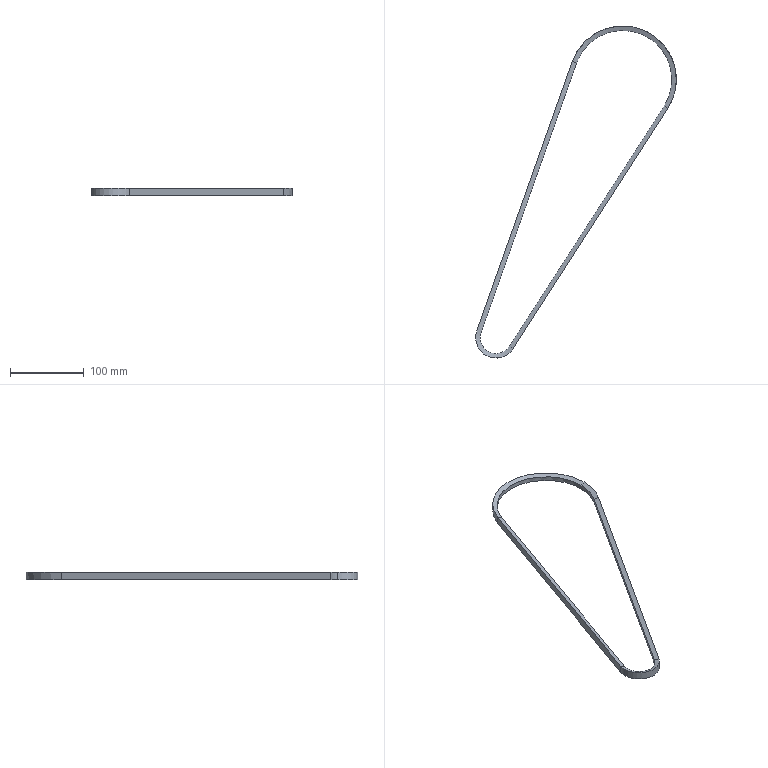Part | SolidWorks | features BaseBody 1 | 1 solid | 20 faces | box 271.5 x 449.339 x 10.319 mm | volume 52741 mm3 | plane 8 | cylinder 6 | cone 6 | commonest cylinder face diameters 42.997 x2 54.997 x2 132.997 x1 144.997 x1
STEP:
#1=CARTESIAN_POINT('',(-148.385,-364.233,5.159));
#2=VERTEX_POINT('',#1);
#3=CARTESIAN_POINT('',(-199.001,-349.342,5.159));
#4=VERTEX_POINT('',#3);
#5=CARTESIAN_POINT('',(-171.503,-349.342,5.159));
#6=DIRECTION('',(0.,0.,-1.));
#7=DIRECTION('',(-1.,0.,0.));
#8=AXIS2_PLACEMENT_3D('',#5,#6,#7);
#9=CIRCLE('',#8,27.499);
#10=EDGE_CURVE('',#2,#4,#9,.T.);
#11=ORIENTED_EDGE('',*,*,#10,.T.);
#12=CARTESIAN_POINT('',(-199.001,-349.342,-5.159));
#13=VERTEX_POINT('',#12);
#14=CARTESIAN_POINT('',(-199.001,-349.342,0.));
#15=DIRECTION('',(0.,0.,-1.));
#16=VECTOR('',#15,1000.);
#17=LINE('',#14,#16);
#18=EDGE_CURVE('',#4,#13,#17,.T.);
#19=ORIENTED_EDGE('',*,*,#18,.T.);
#20=CARTESIAN_POINT('',(-148.385,-364.233,-5.159));
#21=VERTEX_POINT('',#20);
#22=CARTESIAN_POINT('',(-171.503,-349.342,-5.159));
#23=DIRECTION('',(0.,0.,1.));
#24=DIRECTION('',(-1.,0.,0.));
#25=AXIS2_PLACEMENT_3D('',#22,#23,#24);
#26=CIRCLE('',#25,27.499);
#27=EDGE_CURVE('',#13,#21,#26,.T.);
#28=ORIENTED_EDGE('',*,*,#27,.T.);
#29=CARTESIAN_POINT('',(-148.385,-364.233,5.159));
#30=DIRECTION('',(0.,0.,-1.));
#31=VECTOR('',#30,1000.);
#32=LINE('',#29,#31);
#33=EDGE_CURVE('',#2,#21,#32,.T.);
#34=ORIENTED_EDGE('',*,*,#33,.F.);
#35=EDGE_LOOP('',(#11,#19,#28,#34));
#36=FACE_OUTER_BOUND('',#35,.T.);
#37=CARTESIAN_POINT('',(-171.503,-349.342,0.));
#38=DIRECTION('',(0.,0.,-1.));
#39=DIRECTION('',(-1.,0.,0.));
#40=AXIS2_PLACEMENT_3D('',#37,#38,#39);
#41=CYLINDRICAL_SURFACE('',#40,27.499);
#42=ADVANCED_FACE('',(#36),#41,.T.);
#43=CARTESIAN_POINT('',(66.499,0.,2.976));
#44=VERTEX_POINT('',#43);
#45=CARTESIAN_POINT('',(-62.681,22.206,2.976));
#46=VERTEX_POINT('',#45);
#47=CARTESIAN_POINT('',(0.,0.,2.976));
#48=DIRECTION('',(0.,0.,1.));
#49=DIRECTION('',(-0.8407,0.5415,0.));
#50=AXIS2_PLACEMENT_3D('',#47,#48,#49);
#51=CIRCLE('',#50,66.499);
#52=EDGE_CURVE('',#44,#46,#51,.T.);
#53=ORIENTED_EDGE('',*,*,#52,.F.);
#54=CARTESIAN_POINT('',(72.499,0.,5.159));
#55=VERTEX_POINT('',#54);
#56=CARTESIAN_POINT('',(72.499,0.,5.159));
#57=DIRECTION('',(0.9397,0.,0.342));
#58=VECTOR('',#57,1000.);
#59=LINE('',#56,#58);
#60=EDGE_CURVE('',#44,#55,#59,.T.);
#61=ORIENTED_EDGE('',*,*,#60,.T.);
#62=CARTESIAN_POINT('',(-68.337,24.21,5.159));
#63=VERTEX_POINT('',#62);
#64=CARTESIAN_POINT('',(0.,0.,5.159));
#65=DIRECTION('',(0.,0.,-1.));
#66=DIRECTION('',(-1.,0.,0.));
#67=AXIS2_PLACEMENT_3D('',#64,#65,#66);
#68=CIRCLE('',#67,72.499);
#69=EDGE_CURVE('',#63,#55,#68,.T.);
#70=ORIENTED_EDGE('',*,*,#69,.F.);
#71=CARTESIAN_POINT('',(-65.509,23.208,4.068));
#72=DIRECTION('',(-0.8858,0.3138,0.342));
#73=VECTOR('',#72,1000.);
#74=LINE('',#71,#73);
#75=EDGE_CURVE('',#46,#63,#74,.T.);
#76=ORIENTED_EDGE('',*,*,#75,.F.);
#77=EDGE_LOOP('',(#53,#61,#70,#76));
#78=FACE_OUTER_BOUND('',#77,.T.);
#79=CARTESIAN_POINT('',(0.,0.,5.159));
#80=DIRECTION('',(0.,0.,1.));
#81=DIRECTION('',(1.,0.,0.));
#82=AXIS2_PLACEMENT_3D('',#79,#80,#81);
#83=CONICAL_SURFACE('',#82,72.499,1.222);
#84=ADVANCED_FACE('',(#78),#83,.F.);
#85=CARTESIAN_POINT('',(-193.001,-349.342,-2.976));
#86=VERTEX_POINT('',#85);
#87=CARTESIAN_POINT('',(-191.767,-342.163,-2.976));
#88=VERTEX_POINT('',#87);
#89=CARTESIAN_POINT('',(-171.503,-349.342,-2.976));
#90=DIRECTION('',(0.,0.,-1.));
#91=DIRECTION('',(0.9426,-0.3339,0.));
#92=AXIS2_PLACEMENT_3D('',#89,#90,#91);
#93=CIRCLE('',#92,21.499);
#94=EDGE_CURVE('',#86,#88,#93,.T.);
#95=ORIENTED_EDGE('',*,*,#94,.F.);
#96=CARTESIAN_POINT('',(-199.001,-349.342,-5.159));
#97=DIRECTION('',(-0.9397,0.,-0.342));
#98=VECTOR('',#97,1000.);
#99=LINE('',#96,#98);
#100=EDGE_CURVE('',#86,#13,#99,.T.);
#101=ORIENTED_EDGE('',*,*,#100,.T.);
#102=CARTESIAN_POINT('',(-197.423,-340.159,-5.159));
#103=VERTEX_POINT('',#102);
#104=CARTESIAN_POINT('',(-171.503,-349.342,-5.159));
#105=DIRECTION('',(0.,0.,1.));
#106=DIRECTION('',(-1.,0.,0.));
#107=AXIS2_PLACEMENT_3D('',#104,#105,#106);
#108=CIRCLE('',#107,27.499);
#109=EDGE_CURVE('',#103,#13,#108,.T.);
#110=ORIENTED_EDGE('',*,*,#109,.F.);
#111=CARTESIAN_POINT('',(-194.595,-341.161,-4.068));
#112=DIRECTION('',(-0.8858,0.3138,-0.342));
#113=VECTOR('',#112,1000.);
#114=LINE('',#111,#113);
#115=EDGE_CURVE('',#88,#103,#114,.T.);
#116=ORIENTED_EDGE('',*,*,#115,.F.);
#117=EDGE_LOOP('',(#95,#101,#110,#116));
#118=FACE_OUTER_BOUND('',#117,.T.);
#119=CARTESIAN_POINT('',(-171.503,-349.342,-5.159));
#120=DIRECTION('',(0.,0.,-1.));
#121=DIRECTION('',(-1.,0.,0.));
#122=AXIS2_PLACEMENT_3D('',#119,#120,#121);
#123=CONICAL_SURFACE('',#122,27.499,1.222);
#124=ADVANCED_FACE('',(#118),#123,.F.);
#125=CARTESIAN_POINT('',(-191.767,-342.163,2.976));
#126=VERTEX_POINT('',#125);
#127=CARTESIAN_POINT('',(-193.001,-349.342,2.976));
#128=VERTEX_POINT('',#127);
#129=CARTESIAN_POINT('',(-171.503,-349.342,2.976));
#130=DIRECTION('',(0.,0.,1.));
#131=DIRECTION('',(0.9426,-0.3339,0.));
#132=AXIS2_PLACEMENT_3D('',#129,#130,#131);
#133=CIRCLE('',#132,21.499);
#134=EDGE_CURVE('',#126,#128,#133,.T.);
#135=ORIENTED_EDGE('',*,*,#134,.T.);
#136=CARTESIAN_POINT('',(-193.001,-349.342,0.));
#137=DIRECTION('',(0.,0.,-1.));
#138=VECTOR('',#137,1000.);
#139=LINE('',#136,#138);
#140=EDGE_CURVE('',#128,#86,#139,.T.);
#141=ORIENTED_EDGE('',*,*,#140,.T.);
#142=ORIENTED_EDGE('',*,*,#94,.T.);
#143=CARTESIAN_POINT('',(-191.767,-342.163,0.));
#144=DIRECTION('',(0.,0.,-1.));
#145=VECTOR('',#144,1000.);
#146=LINE('',#143,#145);
#147=EDGE_CURVE('',#126,#88,#146,.T.);
#148=ORIENTED_EDGE('',*,*,#147,.F.);
#149=EDGE_LOOP('',(#135,#141,#142,#148));
#150=FACE_OUTER_BOUND('',#149,.T.);
#151=CARTESIAN_POINT('',(-171.503,-349.342,0.));
#152=DIRECTION('',(0.,0.,-1.));
#153=DIRECTION('',(-1.,0.,0.));
#154=AXIS2_PLACEMENT_3D('',#151,#152,#153);
#155=CYLINDRICAL_SURFACE('',#154,21.499);
#156=ADVANCED_FACE('',(#150),#155,.F.);
#157=CARTESIAN_POINT('',(60.948,-39.26,-5.159));
#158=VERTEX_POINT('',#157);
#159=CARTESIAN_POINT('',(60.948,-39.26,5.159));
#160=VERTEX_POINT('',#159);
#161=CARTESIAN_POINT('',(60.948,-39.26,5.159));
#162=DIRECTION('',(0.,0.,1.));
#163=VECTOR('',#162,1000.);
#164=LINE('',#161,#163);
#165=EDGE_CURVE('',#158,#160,#164,.T.);
#166=ORIENTED_EDGE('',*,*,#165,.T.);
#167=CARTESIAN_POINT('',(60.948,-39.26,5.159));
#168=DIRECTION('',(-0.5415,-0.8407,0.));
#169=VECTOR('',#168,1000.);
#170=LINE('',#167,#169);
#171=EDGE_CURVE('',#160,#2,#170,.T.);
#172=ORIENTED_EDGE('',*,*,#171,.T.);
#173=ORIENTED_EDGE('',*,*,#33,.T.);
#174=CARTESIAN_POINT('',(60.948,-39.26,-5.159));
#175=DIRECTION('',(0.5415,0.8407,0.));
#176=VECTOR('',#175,1000.);
#177=LINE('',#174,#176);
#178=EDGE_CURVE('',#21,#158,#177,.T.);
#179=ORIENTED_EDGE('',*,*,#178,.T.);
#180=EDGE_LOOP('',(#166,#172,#173,#179));
#181=FACE_OUTER_BOUND('',#180,.T.);
#182=CARTESIAN_POINT('',(60.948,-39.26,5.159));
#183=DIRECTION('',(0.8407,-0.5415,0.));
#184=DIRECTION('',(0.5415,0.8407,0.));
#185=AXIS2_PLACEMENT_3D('',#182,#183,#184);
#186=PLANE('',#185);
#187=ADVANCED_FACE('',(#181),#186,.T.);
#188=CARTESIAN_POINT('',(55.904,-36.011,2.976));
#189=VERTEX_POINT('',#188);
#190=CARTESIAN_POINT('',(60.948,-39.26,5.159));
#191=DIRECTION('',(-0.79,0.5089,-0.342));
#192=VECTOR('',#191,1000.);
#193=LINE('',#190,#192);
#194=EDGE_CURVE('',#160,#189,#193,.T.);
#195=ORIENTED_EDGE('',*,*,#194,.T.);
#196=CARTESIAN_POINT('',(-153.429,-360.984,2.976));
#197=VERTEX_POINT('',#196);
#198=CARTESIAN_POINT('',(55.904,-36.011,2.976));
#199=DIRECTION('',(-0.5415,-0.8407,0.));
#200=VECTOR('',#199,1000.);
#201=LINE('',#198,#200);
#202=EDGE_CURVE('',#189,#197,#201,.T.);
#203=ORIENTED_EDGE('',*,*,#202,.T.);
#204=CARTESIAN_POINT('',(-153.429,-360.984,2.976));
#205=DIRECTION('',(0.79,-0.5089,0.342));
#206=VECTOR('',#205,1000.);
#207=LINE('',#204,#206);
#208=EDGE_CURVE('',#197,#2,#207,.T.);
#209=ORIENTED_EDGE('',*,*,#208,.T.);
#210=ORIENTED_EDGE('',*,*,#171,.F.);
#211=EDGE_LOOP('',(#195,#203,#209,#210));
#212=FACE_OUTER_BOUND('',#211,.T.);
#213=CARTESIAN_POINT('',(55.904,-36.011,2.976));
#214=DIRECTION('',(-0.2875,0.1852,0.9397));
#215=DIRECTION('',(0.9562,0.,0.2926));
#216=AXIS2_PLACEMENT_3D('',#213,#214,#215);
#217=PLANE('',#216);
#218=ADVANCED_FACE('',(#212),#217,.T.);
#219=CARTESIAN_POINT('',(-68.337,24.21,-5.159));
#220=VERTEX_POINT('',#219);
#221=CARTESIAN_POINT('',(-68.337,24.21,0.));
#222=DIRECTION('',(0.,0.,1.));
#223=VECTOR('',#222,1000.);
#224=LINE('',#221,#223);
#225=EDGE_CURVE('',#220,#63,#224,.T.);
#226=ORIENTED_EDGE('',*,*,#225,.T.);
#227=ORIENTED_EDGE('',*,*,#69,.T.);
#228=CARTESIAN_POINT('',(0.,0.,5.159));
#229=DIRECTION('',(0.,0.,-1.));
#230=DIRECTION('',(-1.,0.,0.));
#231=AXIS2_PLACEMENT_3D('',#228,#229,#230);
#232=CIRCLE('',#231,72.499);
#233=EDGE_CURVE('',#55,#160,#232,.T.);
#234=ORIENTED_EDGE('',*,*,#233,.T.);
#235=ORIENTED_EDGE('',*,*,#165,.F.);
#236=CARTESIAN_POINT('',(0.,0.,-5.159));
#237=DIRECTION('',(0.,0.,1.));
#238=DIRECTION('',(-1.,0.,0.));
#239=AXIS2_PLACEMENT_3D('',#236,#237,#238);
#240=CIRCLE('',#239,72.499);
#241=EDGE_CURVE('',#158,#220,#240,.T.);
#242=ORIENTED_EDGE('',*,*,#241,.T.);
#243=EDGE_LOOP('',(#226,#227,#234,#235,#242));
#244=FACE_OUTER_BOUND('',#243,.T.);
#245=CARTESIAN_POINT('',(0.,0.,0.));
#246=DIRECTION('',(0.,0.,-1.));
#247=DIRECTION('',(-1.,0.,0.));
#248=AXIS2_PLACEMENT_3D('',#245,#246,#247);
#249=CYLINDRICAL_SURFACE('',#248,72.499);
#250=ADVANCED_FACE('',(#244),#249,.T.);
#251=CARTESIAN_POINT('',(55.904,-36.011,-2.976));
#252=VERTEX_POINT('',#251);
#253=CARTESIAN_POINT('',(55.904,-36.011,-2.976));
#254=DIRECTION('',(0.79,-0.5089,-0.342));
#255=VECTOR('',#254,1000.);
#256=LINE('',#253,#255);
#257=EDGE_CURVE('',#252,#158,#256,.T.);
#258=ORIENTED_EDGE('',*,*,#257,.T.);
#259=ORIENTED_EDGE('',*,*,#178,.F.);
#260=CARTESIAN_POINT('',(-153.429,-360.984,-2.976));
#261=VERTEX_POINT('',#260);
#262=CARTESIAN_POINT('',(-148.385,-364.233,-5.159));
#263=DIRECTION('',(-0.79,0.5089,0.342));
#264=VECTOR('',#263,1000.);
#265=LINE('',#262,#264);
#266=EDGE_CURVE('',#21,#261,#265,.T.);
#267=ORIENTED_EDGE('',*,*,#266,.T.);
#268=CARTESIAN_POINT('',(-153.429,-360.984,-2.976));
#269=DIRECTION('',(0.5415,0.8407,0.));
#270=VECTOR('',#269,1000.);
#271=LINE('',#268,#270);
#272=EDGE_CURVE('',#261,#252,#271,.T.);
#273=ORIENTED_EDGE('',*,*,#272,.T.);
#274=EDGE_LOOP('',(#258,#259,#267,#273));
#275=FACE_OUTER_BOUND('',#274,.T.);
#276=CARTESIAN_POINT('',(60.948,-39.26,-5.159));
#277=DIRECTION('',(-0.2875,0.1852,-0.9397));
#278=DIRECTION('',(-0.9562,0.,0.2926));
#279=AXIS2_PLACEMENT_3D('',#276,#277,#278);
#280=PLANE('',#279);
#281=ADVANCED_FACE('',(#275),#280,.T.);
#282=ORIENTED_EDGE('',*,*,#18,.F.);
#283=CARTESIAN_POINT('',(-197.423,-340.159,5.159));
#284=VERTEX_POINT('',#283);
#285=CARTESIAN_POINT('',(-171.503,-349.342,5.159));
#286=DIRECTION('',(0.,0.,-1.));
#287=DIRECTION('',(-1.,0.,0.));
#288=AXIS2_PLACEMENT_3D('',#285,#286,#287);
#289=CIRCLE('',#288,27.499);
#290=EDGE_CURVE('',#4,#284,#289,.T.);
#291=ORIENTED_EDGE('',*,*,#290,.T.);
#292=CARTESIAN_POINT('',(-197.423,-340.159,0.));
#293=DIRECTION('',(0.,0.,-1.));
#294=VECTOR('',#293,1000.);
#295=LINE('',#292,#294);
#296=EDGE_CURVE('',#284,#103,#295,.T.);
#297=ORIENTED_EDGE('',*,*,#296,.T.);
#298=ORIENTED_EDGE('',*,*,#109,.T.);
#299=EDGE_LOOP('',(#282,#291,#297,#298));
#300=FACE_OUTER_BOUND('',#299,.T.);
#301=CARTESIAN_POINT('',(-171.503,-349.342,0.));
#302=DIRECTION('',(0.,0.,-1.));
#303=DIRECTION('',(-1.,0.,0.));
#304=AXIS2_PLACEMENT_3D('',#301,#302,#303);
#305=CYLINDRICAL_SURFACE('',#304,27.499);
#306=ADVANCED_FACE('',(#300),#305,.T.);
#307=CARTESIAN_POINT('',(55.904,-36.011,-2.976));
#308=DIRECTION('',(0.,0.,-1.));
#309=VECTOR('',#308,1000.);
#310=LINE('',#307,#309);
#311=EDGE_CURVE('',#189,#252,#310,.T.);
#312=ORIENTED_EDGE('',*,*,#311,.T.);
#313=ORIENTED_EDGE('',*,*,#272,.F.);
#314=CARTESIAN_POINT('',(-153.429,-360.984,-2.976));
#315=DIRECTION('',(0.,0.,1.));
#316=VECTOR('',#315,1000.);
#317=LINE('',#314,#316);
#318=EDGE_CURVE('',#261,#197,#317,.T.);
#319=ORIENTED_EDGE('',*,*,#318,.T.);
#320=ORIENTED_EDGE('',*,*,#202,.F.);
#321=EDGE_LOOP('',(#312,#313,#319,#320));
#322=FACE_OUTER_BOUND('',#321,.T.);
#323=CARTESIAN_POINT('',(55.904,-36.011,-2.976));
#324=DIRECTION('',(-0.8407,0.5415,0.));
#325=DIRECTION('',(-0.5415,-0.8407,0.));
#326=AXIS2_PLACEMENT_3D('',#323,#324,#325);
#327=PLANE('',#326);
#328=ADVANCED_FACE('',(#322),#327,.T.);
#329=ORIENTED_EDGE('',*,*,#60,.F.);
#330=CARTESIAN_POINT('',(0.,0.,2.976));
#331=DIRECTION('',(0.,0.,1.));
#332=DIRECTION('',(-0.8407,0.5415,0.));
#333=AXIS2_PLACEMENT_3D('',#330,#331,#332);
#334=CIRCLE('',#333,66.499);
#335=EDGE_CURVE('',#189,#44,#334,.T.);
#336=ORIENTED_EDGE('',*,*,#335,.F.);
#337=ORIENTED_EDGE('',*,*,#194,.F.);
#338=ORIENTED_EDGE('',*,*,#233,.F.);
#339=EDGE_LOOP('',(#329,#336,#337,#338));
#340=FACE_OUTER_BOUND('',#339,.T.);
#341=CARTESIAN_POINT('',(0.,0.,5.159));
#342=DIRECTION('',(0.,0.,1.));
#343=DIRECTION('',(1.,0.,0.));
#344=AXIS2_PLACEMENT_3D('',#341,#342,#343);
#345=CONICAL_SURFACE('',#344,72.499,1.222);
#346=ADVANCED_FACE('',(#340),#345,.F.);
#347=ORIENTED_EDGE('',*,*,#10,.F.);
#348=ORIENTED_EDGE('',*,*,#208,.F.);
#349=CARTESIAN_POINT('',(-171.503,-349.342,2.976));
#350=DIRECTION('',(0.,0.,1.));
#351=DIRECTION('',(0.9426,-0.3339,0.));
#352=AXIS2_PLACEMENT_3D('',#349,#350,#351);
#353=CIRCLE('',#352,21.499);
#354=EDGE_CURVE('',#128,#197,#353,.T.);
#355=ORIENTED_EDGE('',*,*,#354,.F.);
#356=ORIENTED_EDGE('',*,*,#134,.F.);
#357=CARTESIAN_POINT('',(-194.595,-341.161,4.068));
#358=DIRECTION('',(0.8858,-0.3138,-0.342));
#359=VECTOR('',#358,1000.);
#360=LINE('',#357,#359);
#361=EDGE_CURVE('',#284,#126,#360,.T.);
#362=ORIENTED_EDGE('',*,*,#361,.F.);
#363=ORIENTED_EDGE('',*,*,#290,.F.);
#364=EDGE_LOOP('',(#347,#348,#355,#356,#362,#363));
#365=FACE_OUTER_BOUND('',#364,.T.);
#366=CARTESIAN_POINT('',(-171.503,-349.342,5.159));
#367=DIRECTION('',(0.,0.,1.));
#368=DIRECTION('',(1.,0.,0.));
#369=AXIS2_PLACEMENT_3D('',#366,#367,#368);
#370=CONICAL_SURFACE('',#369,27.499,1.222);
#371=ADVANCED_FACE('',(#365),#370,.F.);
#372=ORIENTED_EDGE('',*,*,#296,.F.);
#373=CARTESIAN_POINT('',(-197.423,-340.159,5.159));
#374=DIRECTION('',(0.3339,0.9426,0.));
#375=VECTOR('',#374,1000.);
#376=LINE('',#373,#375);
#377=EDGE_CURVE('',#284,#63,#376,.T.);
#378=ORIENTED_EDGE('',*,*,#377,.T.);
#379=ORIENTED_EDGE('',*,*,#225,.F.);
#380=CARTESIAN_POINT('',(-197.423,-340.159,-5.159));
#381=DIRECTION('',(-0.3339,-0.9426,0.));
#382=VECTOR('',#381,1000.);
#383=LINE('',#380,#382);
#384=EDGE_CURVE('',#220,#103,#383,.T.);
#385=ORIENTED_EDGE('',*,*,#384,.T.);
#386=EDGE_LOOP('',(#372,#378,#379,#385));
#387=FACE_OUTER_BOUND('',#386,.T.);
#388=CARTESIAN_POINT('',(-197.423,-340.159,5.159));
#389=DIRECTION('',(-0.9426,0.3339,0.));
#390=DIRECTION('',(-0.3339,-0.9426,0.));
#391=AXIS2_PLACEMENT_3D('',#388,#389,#390);
#392=PLANE('',#391);
#393=ADVANCED_FACE('',(#387),#392,.T.);
#394=CARTESIAN_POINT('',(-62.681,22.206,-2.976));
#395=VERTEX_POINT('',#394);
#396=CARTESIAN_POINT('',(0.,0.,-2.976));
#397=DIRECTION('',(0.,0.,-1.));
#398=DIRECTION('',(-0.8407,0.5415,0.));
#399=AXIS2_PLACEMENT_3D('',#396,#397,#398);
#400=CIRCLE('',#399,66.499);
#401=EDGE_CURVE('',#395,#252,#400,.T.);
#402=ORIENTED_EDGE('',*,*,#401,.F.);
#403=CARTESIAN_POINT('',(-65.509,23.208,-4.068));
#404=DIRECTION('',(0.8858,-0.3138,0.342));
#405=VECTOR('',#404,1000.);
#406=LINE('',#403,#405);
#407=EDGE_CURVE('',#220,#395,#406,.T.);
#408=ORIENTED_EDGE('',*,*,#407,.F.);
#409=ORIENTED_EDGE('',*,*,#241,.F.);
#410=ORIENTED_EDGE('',*,*,#257,.F.);
#411=EDGE_LOOP('',(#402,#408,#409,#410));
#412=FACE_OUTER_BOUND('',#411,.T.);
#413=CARTESIAN_POINT('',(0.,0.,-5.159));
#414=DIRECTION('',(0.,0.,-1.));
#415=DIRECTION('',(-1.,0.,0.));
#416=AXIS2_PLACEMENT_3D('',#413,#414,#415);
#417=CONICAL_SURFACE('',#416,72.499,1.222);
#418=ADVANCED_FACE('',(#412),#417,.F.);
#419=ORIENTED_EDGE('',*,*,#100,.F.);
#420=CARTESIAN_POINT('',(-171.503,-349.342,-2.976));
#421=DIRECTION('',(0.,0.,-1.));
#422=DIRECTION('',(0.9426,-0.3339,0.));
#423=AXIS2_PLACEMENT_3D('',#420,#421,#422);
#424=CIRCLE('',#423,21.499);
#425=EDGE_CURVE('',#261,#86,#424,.T.);
#426=ORIENTED_EDGE('',*,*,#425,.F.);
#427=ORIENTED_EDGE('',*,*,#266,.F.);
#428=ORIENTED_EDGE('',*,*,#27,.F.);
#429=EDGE_LOOP('',(#419,#426,#427,#428));
#430=FACE_OUTER_BOUND('',#429,.T.);
#431=CARTESIAN_POINT('',(-171.503,-349.342,-5.159));
#432=DIRECTION('',(0.,0.,-1.));
#433=DIRECTION('',(-1.,0.,0.));
#434=AXIS2_PLACEMENT_3D('',#431,#432,#433);
#435=CONICAL_SURFACE('',#434,27.499,1.222);
#436=ADVANCED_FACE('',(#430),#435,.F.);
#437=ORIENTED_EDGE('',*,*,#335,.T.);
#438=ORIENTED_EDGE('',*,*,#52,.T.);
#439=CARTESIAN_POINT('',(-62.681,22.206,0.));
#440=DIRECTION('',(0.,0.,1.));
#441=VECTOR('',#440,1000.);
#442=LINE('',#439,#441);
#443=EDGE_CURVE('',#395,#46,#442,.T.);
#444=ORIENTED_EDGE('',*,*,#443,.F.);
#445=ORIENTED_EDGE('',*,*,#401,.T.);
#446=ORIENTED_EDGE('',*,*,#311,.F.);
#447=EDGE_LOOP('',(#437,#438,#444,#445,#446));
#448=FACE_OUTER_BOUND('',#447,.T.);
#449=CARTESIAN_POINT('',(0.,0.,0.));
#450=DIRECTION('',(0.,0.,-1.));
#451=DIRECTION('',(-1.,0.,0.));
#452=AXIS2_PLACEMENT_3D('',#449,#450,#451);
#453=CYLINDRICAL_SURFACE('',#452,66.499);
#454=ADVANCED_FACE('',(#448),#453,.F.);
#455=ORIENTED_EDGE('',*,*,#140,.F.);
#456=ORIENTED_EDGE('',*,*,#354,.T.);
#457=ORIENTED_EDGE('',*,*,#318,.F.);
#458=ORIENTED_EDGE('',*,*,#425,.T.);
#459=EDGE_LOOP('',(#455,#456,#457,#458));
#460=FACE_OUTER_BOUND('',#459,.T.);
#461=CARTESIAN_POINT('',(-171.503,-349.342,0.));
#462=DIRECTION('',(0.,0.,-1.));
#463=DIRECTION('',(-1.,0.,0.));
#464=AXIS2_PLACEMENT_3D('',#461,#462,#463);
#465=CYLINDRICAL_SURFACE('',#464,21.499);
#466=ADVANCED_FACE('',(#460),#465,.F.);
#467=ORIENTED_EDGE('',*,*,#361,.T.);
#468=CARTESIAN_POINT('',(-191.767,-342.163,2.976));
#469=DIRECTION('',(0.3339,0.9426,0.));
#470=VECTOR('',#469,1000.);
#471=LINE('',#468,#470);
#472=EDGE_CURVE('',#126,#46,#471,.T.);
#473=ORIENTED_EDGE('',*,*,#472,.T.);
#474=ORIENTED_EDGE('',*,*,#75,.T.);
#475=ORIENTED_EDGE('',*,*,#377,.F.);
#476=EDGE_LOOP('',(#467,#473,#474,#475));
#477=FACE_OUTER_BOUND('',#476,.T.);
#478=CARTESIAN_POINT('',(-191.767,-342.163,2.976));
#479=DIRECTION('',(0.3224,-0.1142,0.9397));
#480=DIRECTION('',(0.9459,0.,-0.3245));
#481=AXIS2_PLACEMENT_3D('',#478,#479,#480);
#482=PLANE('',#481);
#483=ADVANCED_FACE('',(#477),#482,.T.);
#484=ORIENTED_EDGE('',*,*,#115,.T.);
#485=ORIENTED_EDGE('',*,*,#384,.F.);
#486=ORIENTED_EDGE('',*,*,#407,.T.);
#487=CARTESIAN_POINT('',(-62.681,22.206,-2.976));
#488=DIRECTION('',(-0.3339,-0.9426,0.));
#489=VECTOR('',#488,1000.);
#490=LINE('',#487,#489);
#491=EDGE_CURVE('',#395,#88,#490,.T.);
#492=ORIENTED_EDGE('',*,*,#491,.T.);
#493=EDGE_LOOP('',(#484,#485,#486,#492));
#494=FACE_OUTER_BOUND('',#493,.T.);
#495=CARTESIAN_POINT('',(-197.423,-340.159,-5.159));
#496=DIRECTION('',(0.3224,-0.1142,-0.9397));
#497=DIRECTION('',(-0.9459,0.,-0.3245));
#498=AXIS2_PLACEMENT_3D('',#495,#496,#497);
#499=PLANE('',#498);
#500=ADVANCED_FACE('',(#494),#499,.T.);
#501=ORIENTED_EDGE('',*,*,#147,.T.);
#502=ORIENTED_EDGE('',*,*,#491,.F.);
#503=ORIENTED_EDGE('',*,*,#443,.T.);
#504=ORIENTED_EDGE('',*,*,#472,.F.);
#505=EDGE_LOOP('',(#501,#502,#503,#504));
#506=FACE_OUTER_BOUND('',#505,.T.);
#507=CARTESIAN_POINT('',(-191.767,-342.163,-2.976));
#508=DIRECTION('',(0.9426,-0.3339,0.));
#509=DIRECTION('',(0.3339,0.9426,0.));
#510=AXIS2_PLACEMENT_3D('',#507,#508,#509);
#511=PLANE('',#510);
#512=ADVANCED_FACE('',(#506),#511,.T.);
#513=CLOSED_SHELL('',(#42,#84,#124,#156,#187,#218,#250,#281,#306,#328,#346,#371,#393,#418,#436,#454,#466,#483,#500,#512));
#514=MANIFOLD_SOLID_BREP('',#513);
#515=CARTESIAN_POINT('',(0.,0.,0.));
#516=DIRECTION('',(0.,0.,1.));
#517=DIRECTION('',(1.,0.,0.));
#518=AXIS2_PLACEMENT_3D('',#515,#516,#517);
#519=(LENGTH_UNIT()NAMED_UNIT(*)SI_UNIT(.MILLI.,.METRE.));
#520=UNCERTAINTY_MEASURE_WITH_UNIT(LENGTH_MEASURE(0.00001),#519,'','');
#521=(NAMED_UNIT(*)PLANE_ANGLE_UNIT()SI_UNIT($,.RADIAN.));
#522=(NAMED_UNIT(*)SI_UNIT($,.STERADIAN.)SOLID_ANGLE_UNIT());
#523=(GEOMETRIC_REPRESENTATION_CONTEXT(3)GLOBAL_UNCERTAINTY_ASSIGNED_CONTEXT((#520))GLOBAL_UNIT_ASSIGNED_CONTEXT((#519,#521,#522))REPRESENTATION_CONTEXT('',''));
#524=ADVANCED_BREP_SHAPE_REPRESENTATION('',(#514,#518),#523);